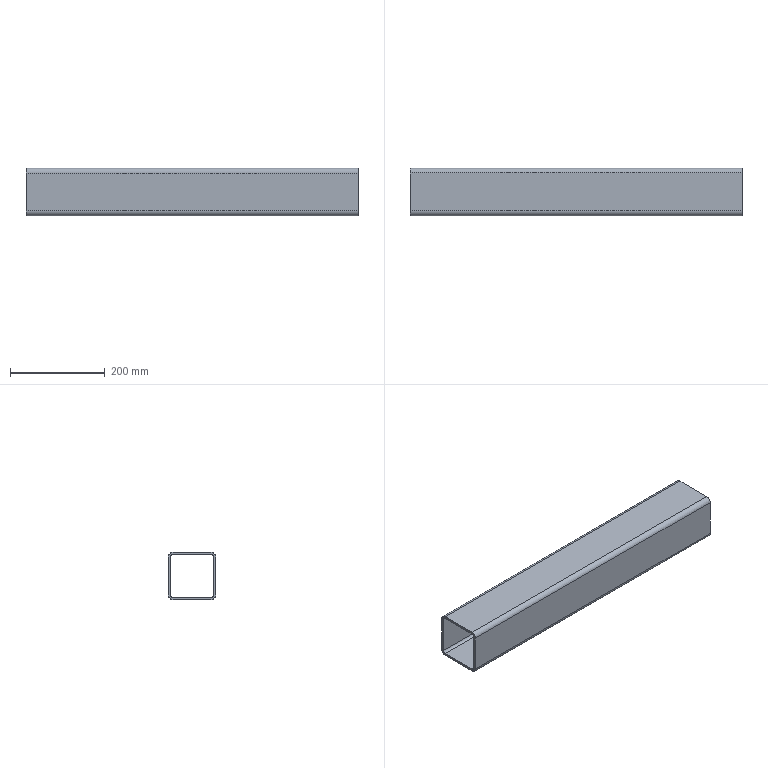Part | SolidWorks | features BaseBody 1 | 1 solid | 18 faces | box 700 x 100 x 100 mm | volume 1284934 mm3 | plane 10 | cylinder 8 | commonest cylinder face diameters 10 x4 20 x4
STEP:
#1=CARTESIAN_POINT('',(-350.,40.,-50.));
#2=VERTEX_POINT('',#1);
#3=CARTESIAN_POINT('',(-350.,50.,-40.));
#4=VERTEX_POINT('',#3);
#5=CARTESIAN_POINT('',(-350.,40.,-40.));
#6=DIRECTION('',(1.,0.,0.));
#7=DIRECTION('',(0.,0.,-1.));
#8=AXIS2_PLACEMENT_3D('',#5,#6,#7);
#9=CIRCLE('',#8,10.);
#10=EDGE_CURVE('',#2,#4,#9,.T.);
#11=ORIENTED_EDGE('',*,*,#10,.T.);
#12=CARTESIAN_POINT('',(350.,50.,-40.));
#13=VERTEX_POINT('',#12);
#14=CARTESIAN_POINT('',(350.,50.,-40.));
#15=DIRECTION('',(-1.,0.,0.));
#16=VECTOR('',#15,1000.);
#17=LINE('',#14,#16);
#18=EDGE_CURVE('',#13,#4,#17,.T.);
#19=ORIENTED_EDGE('',*,*,#18,.F.);
#20=CARTESIAN_POINT('',(350.,40.,-50.));
#21=VERTEX_POINT('',#20);
#22=CARTESIAN_POINT('',(350.,40.,-40.));
#23=DIRECTION('',(1.,0.,0.));
#24=DIRECTION('',(0.,0.,-1.));
#25=AXIS2_PLACEMENT_3D('',#22,#23,#24);
#26=CIRCLE('',#25,10.);
#27=EDGE_CURVE('',#21,#13,#26,.T.);
#28=ORIENTED_EDGE('',*,*,#27,.F.);
#29=CARTESIAN_POINT('',(350.,40.,-50.));
#30=DIRECTION('',(-1.,0.,0.));
#31=VECTOR('',#30,1000.);
#32=LINE('',#29,#31);
#33=EDGE_CURVE('',#21,#2,#32,.T.);
#34=ORIENTED_EDGE('',*,*,#33,.T.);
#35=EDGE_LOOP('',(#11,#19,#28,#34));
#36=FACE_OUTER_BOUND('',#35,.T.);
#37=CARTESIAN_POINT('',(350.,40.,-40.));
#38=DIRECTION('',(-1.,0.,0.));
#39=DIRECTION('',(0.,0.,1.));
#40=AXIS2_PLACEMENT_3D('',#37,#38,#39);
#41=CYLINDRICAL_SURFACE('',#40,10.);
#42=ADVANCED_FACE('',(#36),#41,.T.);
#43=CARTESIAN_POINT('',(-350.,50.,40.));
#44=VERTEX_POINT('',#43);
#45=CARTESIAN_POINT('',(-350.,50.,-40.));
#46=DIRECTION('',(0.,0.,1.));
#47=VECTOR('',#46,1000.);
#48=LINE('',#45,#47);
#49=EDGE_CURVE('',#4,#44,#48,.T.);
#50=ORIENTED_EDGE('',*,*,#49,.T.);
#51=CARTESIAN_POINT('',(350.,50.,40.));
#52=VERTEX_POINT('',#51);
#53=CARTESIAN_POINT('',(350.,50.,40.));
#54=DIRECTION('',(-1.,0.,0.));
#55=VECTOR('',#54,1000.);
#56=LINE('',#53,#55);
#57=EDGE_CURVE('',#52,#44,#56,.T.);
#58=ORIENTED_EDGE('',*,*,#57,.F.);
#59=CARTESIAN_POINT('',(350.,50.,-40.));
#60=DIRECTION('',(0.,0.,1.));
#61=VECTOR('',#60,1000.);
#62=LINE('',#59,#61);
#63=EDGE_CURVE('',#13,#52,#62,.T.);
#64=ORIENTED_EDGE('',*,*,#63,.F.);
#65=ORIENTED_EDGE('',*,*,#18,.T.);
#66=EDGE_LOOP('',(#50,#58,#64,#65));
#67=FACE_OUTER_BOUND('',#66,.T.);
#68=CARTESIAN_POINT('',(350.,50.,-40.));
#69=DIRECTION('',(0.,-1.,0.));
#70=DIRECTION('',(0.,0.,-1.));
#71=AXIS2_PLACEMENT_3D('',#68,#69,#70);
#72=PLANE('',#71);
#73=ADVANCED_FACE('',(#67),#72,.F.);
#74=CARTESIAN_POINT('',(-350.,40.,50.));
#75=VERTEX_POINT('',#74);
#76=CARTESIAN_POINT('',(-350.,40.,40.));
#77=DIRECTION('',(1.,0.,0.));
#78=DIRECTION('',(0.,0.,-1.));
#79=AXIS2_PLACEMENT_3D('',#76,#77,#78);
#80=CIRCLE('',#79,10.);
#81=EDGE_CURVE('',#44,#75,#80,.T.);
#82=ORIENTED_EDGE('',*,*,#81,.T.);
#83=CARTESIAN_POINT('',(350.,40.,50.));
#84=VERTEX_POINT('',#83);
#85=CARTESIAN_POINT('',(350.,40.,50.));
#86=DIRECTION('',(-1.,0.,0.));
#87=VECTOR('',#86,1000.);
#88=LINE('',#85,#87);
#89=EDGE_CURVE('',#84,#75,#88,.T.);
#90=ORIENTED_EDGE('',*,*,#89,.F.);
#91=CARTESIAN_POINT('',(350.,40.,40.));
#92=DIRECTION('',(1.,0.,0.));
#93=DIRECTION('',(0.,0.,-1.));
#94=AXIS2_PLACEMENT_3D('',#91,#92,#93);
#95=CIRCLE('',#94,10.);
#96=EDGE_CURVE('',#52,#84,#95,.T.);
#97=ORIENTED_EDGE('',*,*,#96,.F.);
#98=ORIENTED_EDGE('',*,*,#57,.T.);
#99=EDGE_LOOP('',(#82,#90,#97,#98));
#100=FACE_OUTER_BOUND('',#99,.T.);
#101=CARTESIAN_POINT('',(350.,40.,40.));
#102=DIRECTION('',(-1.,0.,0.));
#103=DIRECTION('',(0.,0.,1.));
#104=AXIS2_PLACEMENT_3D('',#101,#102,#103);
#105=CYLINDRICAL_SURFACE('',#104,10.);
#106=ADVANCED_FACE('',(#100),#105,.T.);
#107=CARTESIAN_POINT('',(-350.,-40.,50.));
#108=VERTEX_POINT('',#107);
#109=CARTESIAN_POINT('',(-350.,-40.,50.));
#110=DIRECTION('',(0.,-1.,0.));
#111=VECTOR('',#110,1000.);
#112=LINE('',#109,#111);
#113=EDGE_CURVE('',#75,#108,#112,.T.);
#114=ORIENTED_EDGE('',*,*,#113,.T.);
#115=CARTESIAN_POINT('',(350.,-40.,50.));
#116=VERTEX_POINT('',#115);
#117=CARTESIAN_POINT('',(350.,-40.,50.));
#118=DIRECTION('',(-1.,0.,0.));
#119=VECTOR('',#118,1000.);
#120=LINE('',#117,#119);
#121=EDGE_CURVE('',#116,#108,#120,.T.);
#122=ORIENTED_EDGE('',*,*,#121,.F.);
#123=CARTESIAN_POINT('',(350.,-40.,50.));
#124=DIRECTION('',(0.,-1.,0.));
#125=VECTOR('',#124,1000.);
#126=LINE('',#123,#125);
#127=EDGE_CURVE('',#84,#116,#126,.T.);
#128=ORIENTED_EDGE('',*,*,#127,.F.);
#129=ORIENTED_EDGE('',*,*,#89,.T.);
#130=EDGE_LOOP('',(#114,#122,#128,#129));
#131=FACE_OUTER_BOUND('',#130,.T.);
#132=CARTESIAN_POINT('',(350.,-40.,50.));
#133=DIRECTION('',(0.,0.,-1.));
#134=DIRECTION('',(0.,1.,0.));
#135=AXIS2_PLACEMENT_3D('',#132,#133,#134);
#136=PLANE('',#135);
#137=ADVANCED_FACE('',(#131),#136,.F.);
#138=CARTESIAN_POINT('',(-350.,-50.,40.));
#139=VERTEX_POINT('',#138);
#140=CARTESIAN_POINT('',(-350.,-40.,40.));
#141=DIRECTION('',(1.,0.,0.));
#142=DIRECTION('',(0.,0.,-1.));
#143=AXIS2_PLACEMENT_3D('',#140,#141,#142);
#144=CIRCLE('',#143,10.);
#145=EDGE_CURVE('',#108,#139,#144,.T.);
#146=ORIENTED_EDGE('',*,*,#145,.T.);
#147=CARTESIAN_POINT('',(350.,-50.,40.));
#148=VERTEX_POINT('',#147);
#149=CARTESIAN_POINT('',(350.,-50.,40.));
#150=DIRECTION('',(-1.,0.,0.));
#151=VECTOR('',#150,1000.);
#152=LINE('',#149,#151);
#153=EDGE_CURVE('',#148,#139,#152,.T.);
#154=ORIENTED_EDGE('',*,*,#153,.F.);
#155=CARTESIAN_POINT('',(350.,-40.,40.));
#156=DIRECTION('',(1.,0.,0.));
#157=DIRECTION('',(0.,0.,-1.));
#158=AXIS2_PLACEMENT_3D('',#155,#156,#157);
#159=CIRCLE('',#158,10.);
#160=EDGE_CURVE('',#116,#148,#159,.T.);
#161=ORIENTED_EDGE('',*,*,#160,.F.);
#162=ORIENTED_EDGE('',*,*,#121,.T.);
#163=EDGE_LOOP('',(#146,#154,#161,#162));
#164=FACE_OUTER_BOUND('',#163,.T.);
#165=CARTESIAN_POINT('',(350.,-40.,40.));
#166=DIRECTION('',(-1.,0.,0.));
#167=DIRECTION('',(0.,0.,1.));
#168=AXIS2_PLACEMENT_3D('',#165,#166,#167);
#169=CYLINDRICAL_SURFACE('',#168,10.);
#170=ADVANCED_FACE('',(#164),#169,.T.);
#171=CARTESIAN_POINT('',(-350.,-50.,-40.));
#172=VERTEX_POINT('',#171);
#173=CARTESIAN_POINT('',(-350.,-50.,40.));
#174=DIRECTION('',(0.,0.,-1.));
#175=VECTOR('',#174,1000.);
#176=LINE('',#173,#175);
#177=EDGE_CURVE('',#139,#172,#176,.T.);
#178=ORIENTED_EDGE('',*,*,#177,.T.);
#179=CARTESIAN_POINT('',(350.,-50.,-40.));
#180=VERTEX_POINT('',#179);
#181=CARTESIAN_POINT('',(350.,-50.,-40.));
#182=DIRECTION('',(-1.,0.,0.));
#183=VECTOR('',#182,1000.);
#184=LINE('',#181,#183);
#185=EDGE_CURVE('',#180,#172,#184,.T.);
#186=ORIENTED_EDGE('',*,*,#185,.F.);
#187=CARTESIAN_POINT('',(350.,-50.,40.));
#188=DIRECTION('',(0.,0.,-1.));
#189=VECTOR('',#188,1000.);
#190=LINE('',#187,#189);
#191=EDGE_CURVE('',#148,#180,#190,.T.);
#192=ORIENTED_EDGE('',*,*,#191,.F.);
#193=ORIENTED_EDGE('',*,*,#153,.T.);
#194=EDGE_LOOP('',(#178,#186,#192,#193));
#195=FACE_OUTER_BOUND('',#194,.T.);
#196=CARTESIAN_POINT('',(350.,-50.,40.));
#197=DIRECTION('',(0.,1.,0.));
#198=DIRECTION('',(0.,0.,1.));
#199=AXIS2_PLACEMENT_3D('',#196,#197,#198);
#200=PLANE('',#199);
#201=ADVANCED_FACE('',(#195),#200,.F.);
#202=CARTESIAN_POINT('',(-350.,-40.,-50.));
#203=VERTEX_POINT('',#202);
#204=CARTESIAN_POINT('',(-350.,-40.,-40.));
#205=DIRECTION('',(1.,0.,0.));
#206=DIRECTION('',(0.,0.,-1.));
#207=AXIS2_PLACEMENT_3D('',#204,#205,#206);
#208=CIRCLE('',#207,10.);
#209=EDGE_CURVE('',#172,#203,#208,.T.);
#210=ORIENTED_EDGE('',*,*,#209,.T.);
#211=CARTESIAN_POINT('',(350.,-40.,-50.));
#212=VERTEX_POINT('',#211);
#213=CARTESIAN_POINT('',(350.,-40.,-50.));
#214=DIRECTION('',(-1.,0.,0.));
#215=VECTOR('',#214,1000.);
#216=LINE('',#213,#215);
#217=EDGE_CURVE('',#212,#203,#216,.T.);
#218=ORIENTED_EDGE('',*,*,#217,.F.);
#219=CARTESIAN_POINT('',(350.,-40.,-40.));
#220=DIRECTION('',(1.,0.,0.));
#221=DIRECTION('',(0.,0.,-1.));
#222=AXIS2_PLACEMENT_3D('',#219,#220,#221);
#223=CIRCLE('',#222,10.);
#224=EDGE_CURVE('',#180,#212,#223,.T.);
#225=ORIENTED_EDGE('',*,*,#224,.F.);
#226=ORIENTED_EDGE('',*,*,#185,.T.);
#227=EDGE_LOOP('',(#210,#218,#225,#226));
#228=FACE_OUTER_BOUND('',#227,.T.);
#229=CARTESIAN_POINT('',(350.,-40.,-40.));
#230=DIRECTION('',(-1.,0.,0.));
#231=DIRECTION('',(0.,0.,1.));
#232=AXIS2_PLACEMENT_3D('',#229,#230,#231);
#233=CYLINDRICAL_SURFACE('',#232,10.);
#234=ADVANCED_FACE('',(#228),#233,.T.);
#235=CARTESIAN_POINT('',(-350.,45.,40.));
#236=VERTEX_POINT('',#235);
#237=CARTESIAN_POINT('',(-350.,40.,45.));
#238=VERTEX_POINT('',#237);
#239=CARTESIAN_POINT('',(-350.,40.,40.));
#240=DIRECTION('',(1.,0.,0.));
#241=DIRECTION('',(0.,0.,-1.));
#242=AXIS2_PLACEMENT_3D('',#239,#240,#241);
#243=CIRCLE('',#242,5.);
#244=EDGE_CURVE('',#236,#238,#243,.T.);
#245=ORIENTED_EDGE('',*,*,#244,.F.);
#246=CARTESIAN_POINT('',(350.,45.,40.));
#247=VERTEX_POINT('',#246);
#248=CARTESIAN_POINT('',(350.,45.,40.));
#249=DIRECTION('',(-1.,0.,0.));
#250=VECTOR('',#249,1000.);
#251=LINE('',#248,#250);
#252=EDGE_CURVE('',#247,#236,#251,.T.);
#253=ORIENTED_EDGE('',*,*,#252,.F.);
#254=CARTESIAN_POINT('',(350.,40.,45.));
#255=VERTEX_POINT('',#254);
#256=CARTESIAN_POINT('',(350.,40.,40.));
#257=DIRECTION('',(1.,0.,0.));
#258=DIRECTION('',(0.,0.,-1.));
#259=AXIS2_PLACEMENT_3D('',#256,#257,#258);
#260=CIRCLE('',#259,5.);
#261=EDGE_CURVE('',#247,#255,#260,.T.);
#262=ORIENTED_EDGE('',*,*,#261,.T.);
#263=CARTESIAN_POINT('',(350.,40.,45.));
#264=DIRECTION('',(-1.,0.,0.));
#265=VECTOR('',#264,1000.);
#266=LINE('',#263,#265);
#267=EDGE_CURVE('',#255,#238,#266,.T.);
#268=ORIENTED_EDGE('',*,*,#267,.T.);
#269=EDGE_LOOP('',(#245,#253,#262,#268));
#270=FACE_OUTER_BOUND('',#269,.T.);
#271=CARTESIAN_POINT('',(350.,40.,40.));
#272=DIRECTION('',(-1.,0.,0.));
#273=DIRECTION('',(0.,0.,1.));
#274=AXIS2_PLACEMENT_3D('',#271,#272,#273);
#275=CYLINDRICAL_SURFACE('',#274,5.);
#276=ADVANCED_FACE('',(#270),#275,.F.);
#277=CARTESIAN_POINT('',(-350.,45.,-40.));
#278=VERTEX_POINT('',#277);
#279=CARTESIAN_POINT('',(-350.,45.,-40.));
#280=DIRECTION('',(0.,0.,1.));
#281=VECTOR('',#280,1000.);
#282=LINE('',#279,#281);
#283=EDGE_CURVE('',#278,#236,#282,.T.);
#284=ORIENTED_EDGE('',*,*,#283,.F.);
#285=CARTESIAN_POINT('',(350.,45.,-40.));
#286=VERTEX_POINT('',#285);
#287=CARTESIAN_POINT('',(350.,45.,-40.));
#288=DIRECTION('',(-1.,0.,0.));
#289=VECTOR('',#288,1000.);
#290=LINE('',#287,#289);
#291=EDGE_CURVE('',#286,#278,#290,.T.);
#292=ORIENTED_EDGE('',*,*,#291,.F.);
#293=CARTESIAN_POINT('',(350.,45.,-40.));
#294=DIRECTION('',(0.,0.,1.));
#295=VECTOR('',#294,1000.);
#296=LINE('',#293,#295);
#297=EDGE_CURVE('',#286,#247,#296,.T.);
#298=ORIENTED_EDGE('',*,*,#297,.T.);
#299=ORIENTED_EDGE('',*,*,#252,.T.);
#300=EDGE_LOOP('',(#284,#292,#298,#299));
#301=FACE_OUTER_BOUND('',#300,.T.);
#302=CARTESIAN_POINT('',(350.,45.,-40.));
#303=DIRECTION('',(0.,-1.,0.));
#304=DIRECTION('',(0.,0.,-1.));
#305=AXIS2_PLACEMENT_3D('',#302,#303,#304);
#306=PLANE('',#305);
#307=ADVANCED_FACE('',(#301),#306,.T.);
#308=CARTESIAN_POINT('',(-350.,40.,-45.));
#309=VERTEX_POINT('',#308);
#310=CARTESIAN_POINT('',(-350.,40.,-40.));
#311=DIRECTION('',(1.,0.,0.));
#312=DIRECTION('',(0.,0.,-1.));
#313=AXIS2_PLACEMENT_3D('',#310,#311,#312);
#314=CIRCLE('',#313,5.);
#315=EDGE_CURVE('',#309,#278,#314,.T.);
#316=ORIENTED_EDGE('',*,*,#315,.F.);
#317=CARTESIAN_POINT('',(350.,40.,-45.));
#318=VERTEX_POINT('',#317);
#319=CARTESIAN_POINT('',(350.,40.,-45.));
#320=DIRECTION('',(-1.,0.,0.));
#321=VECTOR('',#320,1000.);
#322=LINE('',#319,#321);
#323=EDGE_CURVE('',#318,#309,#322,.T.);
#324=ORIENTED_EDGE('',*,*,#323,.F.);
#325=CARTESIAN_POINT('',(350.,40.,-40.));
#326=DIRECTION('',(1.,0.,0.));
#327=DIRECTION('',(0.,0.,-1.));
#328=AXIS2_PLACEMENT_3D('',#325,#326,#327);
#329=CIRCLE('',#328,5.);
#330=EDGE_CURVE('',#318,#286,#329,.T.);
#331=ORIENTED_EDGE('',*,*,#330,.T.);
#332=ORIENTED_EDGE('',*,*,#291,.T.);
#333=EDGE_LOOP('',(#316,#324,#331,#332));
#334=FACE_OUTER_BOUND('',#333,.T.);
#335=CARTESIAN_POINT('',(350.,40.,-40.));
#336=DIRECTION('',(-1.,0.,0.));
#337=DIRECTION('',(0.,0.,1.));
#338=AXIS2_PLACEMENT_3D('',#335,#336,#337);
#339=CYLINDRICAL_SURFACE('',#338,5.);
#340=ADVANCED_FACE('',(#334),#339,.F.);
#341=CARTESIAN_POINT('',(-350.,-40.,-45.));
#342=VERTEX_POINT('',#341);
#343=CARTESIAN_POINT('',(-350.,40.,-45.));
#344=DIRECTION('',(0.,1.,0.));
#345=VECTOR('',#344,1000.);
#346=LINE('',#343,#345);
#347=EDGE_CURVE('',#342,#309,#346,.T.);
#348=ORIENTED_EDGE('',*,*,#347,.F.);
#349=CARTESIAN_POINT('',(350.,-40.,-45.));
#350=VERTEX_POINT('',#349);
#351=CARTESIAN_POINT('',(350.,-40.,-45.));
#352=DIRECTION('',(-1.,0.,0.));
#353=VECTOR('',#352,1000.);
#354=LINE('',#351,#353);
#355=EDGE_CURVE('',#350,#342,#354,.T.);
#356=ORIENTED_EDGE('',*,*,#355,.F.);
#357=CARTESIAN_POINT('',(350.,40.,-45.));
#358=DIRECTION('',(0.,1.,0.));
#359=VECTOR('',#358,1000.);
#360=LINE('',#357,#359);
#361=EDGE_CURVE('',#350,#318,#360,.T.);
#362=ORIENTED_EDGE('',*,*,#361,.T.);
#363=ORIENTED_EDGE('',*,*,#323,.T.);
#364=EDGE_LOOP('',(#348,#356,#362,#363));
#365=FACE_OUTER_BOUND('',#364,.T.);
#366=CARTESIAN_POINT('',(350.,40.,-45.));
#367=DIRECTION('',(0.,0.,1.));
#368=DIRECTION('',(1.,0.,0.));
#369=AXIS2_PLACEMENT_3D('',#366,#367,#368);
#370=PLANE('',#369);
#371=ADVANCED_FACE('',(#365),#370,.T.);
#372=CARTESIAN_POINT('',(-350.,-45.,-40.));
#373=VERTEX_POINT('',#372);
#374=CARTESIAN_POINT('',(-350.,-40.,-40.));
#375=DIRECTION('',(1.,0.,0.));
#376=DIRECTION('',(0.,0.,-1.));
#377=AXIS2_PLACEMENT_3D('',#374,#375,#376);
#378=CIRCLE('',#377,5.);
#379=EDGE_CURVE('',#373,#342,#378,.T.);
#380=ORIENTED_EDGE('',*,*,#379,.F.);
#381=CARTESIAN_POINT('',(350.,-45.,-40.));
#382=VERTEX_POINT('',#381);
#383=CARTESIAN_POINT('',(350.,-45.,-40.));
#384=DIRECTION('',(-1.,0.,0.));
#385=VECTOR('',#384,1000.);
#386=LINE('',#383,#385);
#387=EDGE_CURVE('',#382,#373,#386,.T.);
#388=ORIENTED_EDGE('',*,*,#387,.F.);
#389=CARTESIAN_POINT('',(350.,-40.,-40.));
#390=DIRECTION('',(1.,0.,0.));
#391=DIRECTION('',(0.,0.,-1.));
#392=AXIS2_PLACEMENT_3D('',#389,#390,#391);
#393=CIRCLE('',#392,5.);
#394=EDGE_CURVE('',#382,#350,#393,.T.);
#395=ORIENTED_EDGE('',*,*,#394,.T.);
#396=ORIENTED_EDGE('',*,*,#355,.T.);
#397=EDGE_LOOP('',(#380,#388,#395,#396));
#398=FACE_OUTER_BOUND('',#397,.T.);
#399=CARTESIAN_POINT('',(350.,-40.,-40.));
#400=DIRECTION('',(-1.,0.,0.));
#401=DIRECTION('',(0.,0.,1.));
#402=AXIS2_PLACEMENT_3D('',#399,#400,#401);
#403=CYLINDRICAL_SURFACE('',#402,5.);
#404=ADVANCED_FACE('',(#398),#403,.F.);
#405=CARTESIAN_POINT('',(-350.,-45.,40.));
#406=VERTEX_POINT('',#405);
#407=CARTESIAN_POINT('',(-350.,-45.,40.));
#408=DIRECTION('',(0.,0.,-1.));
#409=VECTOR('',#408,1000.);
#410=LINE('',#407,#409);
#411=EDGE_CURVE('',#406,#373,#410,.T.);
#412=ORIENTED_EDGE('',*,*,#411,.F.);
#413=CARTESIAN_POINT('',(350.,-45.,40.));
#414=VERTEX_POINT('',#413);
#415=CARTESIAN_POINT('',(350.,-45.,40.));
#416=DIRECTION('',(-1.,0.,0.));
#417=VECTOR('',#416,1000.);
#418=LINE('',#415,#417);
#419=EDGE_CURVE('',#414,#406,#418,.T.);
#420=ORIENTED_EDGE('',*,*,#419,.F.);
#421=CARTESIAN_POINT('',(350.,-45.,40.));
#422=DIRECTION('',(0.,0.,-1.));
#423=VECTOR('',#422,1000.);
#424=LINE('',#421,#423);
#425=EDGE_CURVE('',#414,#382,#424,.T.);
#426=ORIENTED_EDGE('',*,*,#425,.T.);
#427=ORIENTED_EDGE('',*,*,#387,.T.);
#428=EDGE_LOOP('',(#412,#420,#426,#427));
#429=FACE_OUTER_BOUND('',#428,.T.);
#430=CARTESIAN_POINT('',(350.,-45.,40.));
#431=DIRECTION('',(0.,1.,0.));
#432=DIRECTION('',(0.,0.,1.));
#433=AXIS2_PLACEMENT_3D('',#430,#431,#432);
#434=PLANE('',#433);
#435=ADVANCED_FACE('',(#429),#434,.T.);
#436=CARTESIAN_POINT('',(-350.,-40.,45.));
#437=VERTEX_POINT('',#436);
#438=CARTESIAN_POINT('',(-350.,-40.,40.));
#439=DIRECTION('',(1.,0.,0.));
#440=DIRECTION('',(0.,0.,-1.));
#441=AXIS2_PLACEMENT_3D('',#438,#439,#440);
#442=CIRCLE('',#441,5.);
#443=EDGE_CURVE('',#437,#406,#442,.T.);
#444=ORIENTED_EDGE('',*,*,#443,.F.);
#445=CARTESIAN_POINT('',(350.,-40.,45.));
#446=VERTEX_POINT('',#445);
#447=CARTESIAN_POINT('',(350.,-40.,45.));
#448=DIRECTION('',(-1.,0.,0.));
#449=VECTOR('',#448,1000.);
#450=LINE('',#447,#449);
#451=EDGE_CURVE('',#446,#437,#450,.T.);
#452=ORIENTED_EDGE('',*,*,#451,.F.);
#453=CARTESIAN_POINT('',(350.,-40.,40.));
#454=DIRECTION('',(1.,0.,0.));
#455=DIRECTION('',(0.,0.,-1.));
#456=AXIS2_PLACEMENT_3D('',#453,#454,#455);
#457=CIRCLE('',#456,5.);
#458=EDGE_CURVE('',#446,#414,#457,.T.);
#459=ORIENTED_EDGE('',*,*,#458,.T.);
#460=ORIENTED_EDGE('',*,*,#419,.T.);
#461=EDGE_LOOP('',(#444,#452,#459,#460));
#462=FACE_OUTER_BOUND('',#461,.T.);
#463=CARTESIAN_POINT('',(350.,-40.,40.));
#464=DIRECTION('',(-1.,0.,0.));
#465=DIRECTION('',(0.,0.,1.));
#466=AXIS2_PLACEMENT_3D('',#463,#464,#465);
#467=CYLINDRICAL_SURFACE('',#466,5.);
#468=ADVANCED_FACE('',(#462),#467,.F.);
#469=CARTESIAN_POINT('',(-350.,-40.,45.));
#470=DIRECTION('',(0.,-1.,0.));
#471=VECTOR('',#470,1000.);
#472=LINE('',#469,#471);
#473=EDGE_CURVE('',#238,#437,#472,.T.);
#474=ORIENTED_EDGE('',*,*,#473,.F.);
#475=ORIENTED_EDGE('',*,*,#267,.F.);
#476=CARTESIAN_POINT('',(350.,-40.,45.));
#477=DIRECTION('',(0.,-1.,0.));
#478=VECTOR('',#477,1000.);
#479=LINE('',#476,#478);
#480=EDGE_CURVE('',#255,#446,#479,.T.);
#481=ORIENTED_EDGE('',*,*,#480,.T.);
#482=ORIENTED_EDGE('',*,*,#451,.T.);
#483=EDGE_LOOP('',(#474,#475,#481,#482));
#484=FACE_OUTER_BOUND('',#483,.T.);
#485=CARTESIAN_POINT('',(350.,-40.,45.));
#486=DIRECTION('',(0.,0.,-1.));
#487=DIRECTION('',(0.,1.,0.));
#488=AXIS2_PLACEMENT_3D('',#485,#486,#487);
#489=PLANE('',#488);
#490=ADVANCED_FACE('',(#484),#489,.T.);
#491=CARTESIAN_POINT('',(-350.,40.,-50.));
#492=DIRECTION('',(0.,1.,0.));
#493=VECTOR('',#492,1000.);
#494=LINE('',#491,#493);
#495=EDGE_CURVE('',#203,#2,#494,.T.);
#496=ORIENTED_EDGE('',*,*,#495,.T.);
#497=ORIENTED_EDGE('',*,*,#33,.F.);
#498=CARTESIAN_POINT('',(350.,40.,-50.));
#499=DIRECTION('',(0.,1.,0.));
#500=VECTOR('',#499,1000.);
#501=LINE('',#498,#500);
#502=EDGE_CURVE('',#212,#21,#501,.T.);
#503=ORIENTED_EDGE('',*,*,#502,.F.);
#504=ORIENTED_EDGE('',*,*,#217,.T.);
#505=EDGE_LOOP('',(#496,#497,#503,#504));
#506=FACE_OUTER_BOUND('',#505,.T.);
#507=CARTESIAN_POINT('',(350.,40.,-50.));
#508=DIRECTION('',(0.,0.,1.));
#509=DIRECTION('',(1.,0.,0.));
#510=AXIS2_PLACEMENT_3D('',#507,#508,#509);
#511=PLANE('',#510);
#512=ADVANCED_FACE('',(#506),#511,.F.);
#513=ORIENTED_EDGE('',*,*,#261,.F.);
#514=ORIENTED_EDGE('',*,*,#297,.F.);
#515=ORIENTED_EDGE('',*,*,#330,.F.);
#516=ORIENTED_EDGE('',*,*,#361,.F.);
#517=ORIENTED_EDGE('',*,*,#394,.F.);
#518=ORIENTED_EDGE('',*,*,#425,.F.);
#519=ORIENTED_EDGE('',*,*,#458,.F.);
#520=ORIENTED_EDGE('',*,*,#480,.F.);
#521=EDGE_LOOP('',(#513,#514,#515,#516,#517,#518,#519,#520));
#522=FACE_BOUND('',#521,.T.);
#523=ORIENTED_EDGE('',*,*,#27,.T.);
#524=ORIENTED_EDGE('',*,*,#63,.T.);
#525=ORIENTED_EDGE('',*,*,#96,.T.);
#526=ORIENTED_EDGE('',*,*,#127,.T.);
#527=ORIENTED_EDGE('',*,*,#160,.T.);
#528=ORIENTED_EDGE('',*,*,#191,.T.);
#529=ORIENTED_EDGE('',*,*,#224,.T.);
#530=ORIENTED_EDGE('',*,*,#502,.T.);
#531=EDGE_LOOP('',(#523,#524,#525,#526,#527,#528,#529,#530));
#532=FACE_OUTER_BOUND('',#531,.T.);
#533=CARTESIAN_POINT('',(350.,40.,-40.));
#534=DIRECTION('',(1.,0.,0.));
#535=DIRECTION('',(0.,0.,-1.));
#536=AXIS2_PLACEMENT_3D('',#533,#534,#535);
#537=PLANE('',#536);
#538=ADVANCED_FACE('',(#522,#532),#537,.T.);
#539=ORIENTED_EDGE('',*,*,#244,.T.);
#540=ORIENTED_EDGE('',*,*,#473,.T.);
#541=ORIENTED_EDGE('',*,*,#443,.T.);
#542=ORIENTED_EDGE('',*,*,#411,.T.);
#543=ORIENTED_EDGE('',*,*,#379,.T.);
#544=ORIENTED_EDGE('',*,*,#347,.T.);
#545=ORIENTED_EDGE('',*,*,#315,.T.);
#546=ORIENTED_EDGE('',*,*,#283,.T.);
#547=EDGE_LOOP('',(#539,#540,#541,#542,#543,#544,#545,#546));
#548=FACE_BOUND('',#547,.T.);
#549=ORIENTED_EDGE('',*,*,#10,.F.);
#550=ORIENTED_EDGE('',*,*,#495,.F.);
#551=ORIENTED_EDGE('',*,*,#209,.F.);
#552=ORIENTED_EDGE('',*,*,#177,.F.);
#553=ORIENTED_EDGE('',*,*,#145,.F.);
#554=ORIENTED_EDGE('',*,*,#113,.F.);
#555=ORIENTED_EDGE('',*,*,#81,.F.);
#556=ORIENTED_EDGE('',*,*,#49,.F.);
#557=EDGE_LOOP('',(#549,#550,#551,#552,#553,#554,#555,#556));
#558=FACE_OUTER_BOUND('',#557,.T.);
#559=CARTESIAN_POINT('',(-350.,40.,-40.));
#560=DIRECTION('',(1.,0.,0.));
#561=DIRECTION('',(0.,0.,-1.));
#562=AXIS2_PLACEMENT_3D('',#559,#560,#561);
#563=PLANE('',#562);
#564=ADVANCED_FACE('',(#548,#558),#563,.F.);
#565=CLOSED_SHELL('',(#42,#73,#106,#137,#170,#201,#234,#276,#307,#340,#371,#404,#435,#468,#490,#512,#538,#564));
#566=MANIFOLD_SOLID_BREP('',#565);
#567=CARTESIAN_POINT('',(0.,0.,0.));
#568=DIRECTION('',(0.,0.,1.));
#569=DIRECTION('',(1.,0.,0.));
#570=AXIS2_PLACEMENT_3D('',#567,#568,#569);
#571=(LENGTH_UNIT()NAMED_UNIT(*)SI_UNIT(.MILLI.,.METRE.));
#572=UNCERTAINTY_MEASURE_WITH_UNIT(LENGTH_MEASURE(0.00001),#571,'','');
#573=(NAMED_UNIT(*)PLANE_ANGLE_UNIT()SI_UNIT($,.RADIAN.));
#574=(NAMED_UNIT(*)SI_UNIT($,.STERADIAN.)SOLID_ANGLE_UNIT());
#575=(GEOMETRIC_REPRESENTATION_CONTEXT(3)GLOBAL_UNCERTAINTY_ASSIGNED_CONTEXT((#572))GLOBAL_UNIT_ASSIGNED_CONTEXT((#571,#573,#574))REPRESENTATION_CONTEXT('',''));
#576=ADVANCED_BREP_SHAPE_REPRESENTATION('',(#566,#570),#575);